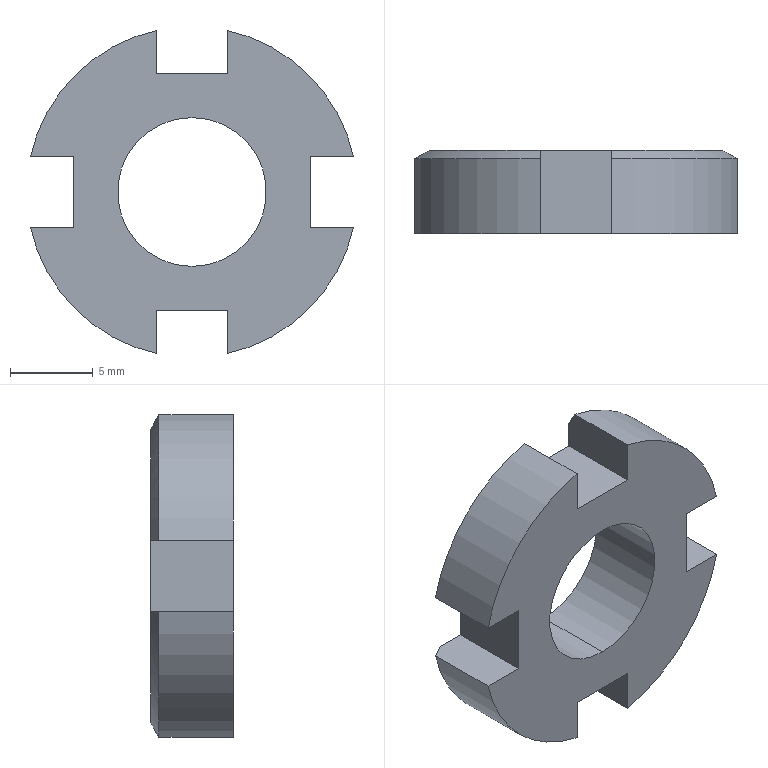Part | SolidWorks | features Chamfer 1, Extrusion 1, HoleWzd 1 | 1 solid | 24 faces | box 19.532 x 5 x 19.532 mm | volume 1006 mm3 | plane 14 | cylinder 6 | cone 4 | commonest cylinder face diameters 20 x4 9 x2
STEP:
#1=CARTESIAN_POINT('',(0.,0.,-4.5));
#2=VERTEX_POINT('',#1);
#3=CARTESIAN_POINT('',(0.,0.,4.5));
#4=VERTEX_POINT('',#3);
#5=CARTESIAN_POINT('',(0.,0.,0.));
#6=DIRECTION('',(0.,1.,0.));
#7=DIRECTION('',(0.,0.,1.));
#8=AXIS2_PLACEMENT_3D('',#5,#6,#7);
#9=CIRCLE('',#8,4.5);
#10=EDGE_CURVE('',#2,#4,#9,.T.);
#11=ORIENTED_EDGE('',*,*,#10,.F.);
#12=CARTESIAN_POINT('',(0.,5.,-4.5));
#13=VERTEX_POINT('',#12);
#14=CARTESIAN_POINT('',(0.,5.,-4.5));
#15=DIRECTION('',(0.,1.,0.));
#16=VECTOR('',#15,1000.);
#17=LINE('',#14,#16);
#18=EDGE_CURVE('',#2,#13,#17,.T.);
#19=ORIENTED_EDGE('',*,*,#18,.T.);
#20=CARTESIAN_POINT('',(0.,5.,4.5));
#21=VERTEX_POINT('',#20);
#22=CARTESIAN_POINT('',(0.,5.,0.));
#23=DIRECTION('',(0.,1.,0.));
#24=DIRECTION('',(0.,0.,1.));
#25=AXIS2_PLACEMENT_3D('',#22,#23,#24);
#26=CIRCLE('',#25,4.5);
#27=EDGE_CURVE('',#13,#21,#26,.T.);
#28=ORIENTED_EDGE('',*,*,#27,.T.);
#29=CARTESIAN_POINT('',(0.,5.,4.5));
#30=DIRECTION('',(0.,1.,0.));
#31=VECTOR('',#30,1000.);
#32=LINE('',#29,#31);
#33=EDGE_CURVE('',#4,#21,#32,.T.);
#34=ORIENTED_EDGE('',*,*,#33,.F.);
#35=EDGE_LOOP('',(#11,#19,#28,#34));
#36=FACE_OUTER_BOUND('',#35,.T.);
#37=CARTESIAN_POINT('',(0.,5.,0.));
#38=DIRECTION('',(0.,1.,0.));
#39=DIRECTION('',(0.,0.,1.));
#40=AXIS2_PLACEMENT_3D('',#37,#38,#39);
#41=CYLINDRICAL_SURFACE('',#40,4.5);
#42=ADVANCED_FACE('',(#36),#41,.F.);
#43=CARTESIAN_POINT('',(-9.766,4.5,-2.15));
#44=VERTEX_POINT('',#43);
#45=CARTESIAN_POINT('',(-9.766,0.,-2.15));
#46=VERTEX_POINT('',#45);
#47=CARTESIAN_POINT('',(-9.766,5.,-2.15));
#48=DIRECTION('',(0.,-1.,0.));
#49=VECTOR('',#48,1000.);
#50=LINE('',#47,#49);
#51=EDGE_CURVE('',#44,#46,#50,.T.);
#52=ORIENTED_EDGE('',*,*,#51,.F.);
#53=CARTESIAN_POINT('',(-2.15,4.5,-9.766));
#54=VERTEX_POINT('',#53);
#55=CARTESIAN_POINT('',(0.,4.5,0.));
#56=DIRECTION('',(0.,-1.,0.));
#57=DIRECTION('',(0.,0.,1.));
#58=AXIS2_PLACEMENT_3D('',#55,#56,#57);
#59=CIRCLE('',#58,10.);
#60=EDGE_CURVE('',#44,#54,#59,.T.);
#61=ORIENTED_EDGE('',*,*,#60,.T.);
#62=CARTESIAN_POINT('',(-2.15,0.,-9.766));
#63=VERTEX_POINT('',#62);
#64=CARTESIAN_POINT('',(-2.15,5.,-9.766));
#65=DIRECTION('',(0.,-1.,0.));
#66=VECTOR('',#65,1000.);
#67=LINE('',#64,#66);
#68=EDGE_CURVE('',#54,#63,#67,.T.);
#69=ORIENTED_EDGE('',*,*,#68,.T.);
#70=CARTESIAN_POINT('',(0.,0.,0.));
#71=DIRECTION('',(0.,1.,0.));
#72=DIRECTION('',(0.,0.,1.));
#73=AXIS2_PLACEMENT_3D('',#70,#71,#72);
#74=CIRCLE('',#73,10.);
#75=EDGE_CURVE('',#63,#46,#74,.T.);
#76=ORIENTED_EDGE('',*,*,#75,.T.);
#77=EDGE_LOOP('',(#52,#61,#69,#76));
#78=FACE_OUTER_BOUND('',#77,.T.);
#79=CARTESIAN_POINT('',(0.,5.,0.));
#80=DIRECTION('',(0.,-1.,0.));
#81=DIRECTION('',(0.,0.,-1.));
#82=AXIS2_PLACEMENT_3D('',#79,#80,#81);
#83=CYLINDRICAL_SURFACE('',#82,10.);
#84=ADVANCED_FACE('',(#78),#83,.T.);
#85=CARTESIAN_POINT('',(-8.877,5.,-2.15));
#86=VERTEX_POINT('',#85);
#87=CARTESIAN_POINT('',(-7.166,5.,-2.15));
#88=VERTEX_POINT('',#87);
#89=CARTESIAN_POINT('',(-7.166,5.,-2.15));
#90=DIRECTION('',(1.,0.,0.));
#91=VECTOR('',#90,1000.);
#92=LINE('',#89,#91);
#93=EDGE_CURVE('',#86,#88,#92,.T.);
#94=ORIENTED_EDGE('',*,*,#93,.F.);
#95=CARTESIAN_POINT('',(-8.877,5.,-2.15));
#96=CARTESIAN_POINT('',(-9.174,4.834,-2.15));
#97=CARTESIAN_POINT('',(-9.47,4.667,-2.15));
#98=CARTESIAN_POINT('',(-9.766,4.5,-2.15));
#99=B_SPLINE_CURVE_WITH_KNOTS('',3,(#95,#96,#97,#98),.UNSPECIFIED.,.F.,.F.,(4,4),(0.,0.00102),.UNSPECIFIED.);
#100=EDGE_CURVE('',#86,#44,#99,.T.);
#101=ORIENTED_EDGE('',*,*,#100,.T.);
#102=ORIENTED_EDGE('',*,*,#51,.T.);
#103=CARTESIAN_POINT('',(-7.166,0.,-2.15));
#104=VERTEX_POINT('',#103);
#105=CARTESIAN_POINT('',(-7.166,0.,-2.15));
#106=DIRECTION('',(1.,0.,0.));
#107=VECTOR('',#106,1000.);
#108=LINE('',#105,#107);
#109=EDGE_CURVE('',#46,#104,#108,.T.);
#110=ORIENTED_EDGE('',*,*,#109,.T.);
#111=CARTESIAN_POINT('',(-7.166,5.,-2.15));
#112=DIRECTION('',(0.,-1.,0.));
#113=VECTOR('',#112,1000.);
#114=LINE('',#111,#113);
#115=EDGE_CURVE('',#88,#104,#114,.T.);
#116=ORIENTED_EDGE('',*,*,#115,.F.);
#117=EDGE_LOOP('',(#94,#101,#102,#110,#116));
#118=FACE_OUTER_BOUND('',#117,.T.);
#119=CARTESIAN_POINT('',(-7.166,5.,-2.15));
#120=DIRECTION('',(0.,0.,-1.));
#121=DIRECTION('',(-1.,0.,0.));
#122=AXIS2_PLACEMENT_3D('',#119,#120,#121);
#123=PLANE('',#122);
#124=ADVANCED_FACE('',(#118),#123,.F.);
#125=CARTESIAN_POINT('',(-7.166,0.,2.15));
#126=VERTEX_POINT('',#125);
#127=CARTESIAN_POINT('',(-7.166,0.,2.15));
#128=DIRECTION('',(0.,0.,1.));
#129=VECTOR('',#128,1000.);
#130=LINE('',#127,#129);
#131=EDGE_CURVE('',#104,#126,#130,.T.);
#132=ORIENTED_EDGE('',*,*,#131,.T.);
#133=CARTESIAN_POINT('',(-7.166,5.,2.15));
#134=VERTEX_POINT('',#133);
#135=CARTESIAN_POINT('',(-7.166,5.,2.15));
#136=DIRECTION('',(0.,-1.,0.));
#137=VECTOR('',#136,1000.);
#138=LINE('',#135,#137);
#139=EDGE_CURVE('',#134,#126,#138,.T.);
#140=ORIENTED_EDGE('',*,*,#139,.F.);
#141=CARTESIAN_POINT('',(-7.166,5.,2.15));
#142=DIRECTION('',(0.,0.,1.));
#143=VECTOR('',#142,1000.);
#144=LINE('',#141,#143);
#145=EDGE_CURVE('',#88,#134,#144,.T.);
#146=ORIENTED_EDGE('',*,*,#145,.F.);
#147=ORIENTED_EDGE('',*,*,#115,.T.);
#148=EDGE_LOOP('',(#132,#140,#146,#147));
#149=FACE_OUTER_BOUND('',#148,.T.);
#150=CARTESIAN_POINT('',(-7.166,5.,2.15));
#151=DIRECTION('',(1.,0.,0.));
#152=DIRECTION('',(0.,0.,-1.));
#153=AXIS2_PLACEMENT_3D('',#150,#151,#152);
#154=PLANE('',#153);
#155=ADVANCED_FACE('',(#149),#154,.F.);
#156=CARTESIAN_POINT('',(-9.766,4.5,2.15));
#157=VERTEX_POINT('',#156);
#158=CARTESIAN_POINT('',(-9.766,0.,2.15));
#159=VERTEX_POINT('',#158);
#160=CARTESIAN_POINT('',(-9.766,5.,2.15));
#161=DIRECTION('',(0.,-1.,0.));
#162=VECTOR('',#161,1000.);
#163=LINE('',#160,#162);
#164=EDGE_CURVE('',#157,#159,#163,.T.);
#165=ORIENTED_EDGE('',*,*,#164,.F.);
#166=CARTESIAN_POINT('',(-8.877,5.,2.15));
#167=VERTEX_POINT('',#166);
#168=CARTESIAN_POINT('',(-9.766,4.5,2.15));
#169=CARTESIAN_POINT('',(-9.47,4.667,2.15));
#170=CARTESIAN_POINT('',(-9.174,4.834,2.15));
#171=CARTESIAN_POINT('',(-8.877,5.,2.15));
#172=B_SPLINE_CURVE_WITH_KNOTS('',3,(#168,#169,#170,#171),.UNSPECIFIED.,.F.,.F.,(4,4),(0.,0.00102),.UNSPECIFIED.);
#173=EDGE_CURVE('',#157,#167,#172,.T.);
#174=ORIENTED_EDGE('',*,*,#173,.T.);
#175=CARTESIAN_POINT('',(-9.766,5.,2.15));
#176=DIRECTION('',(-1.,0.,0.));
#177=VECTOR('',#176,1000.);
#178=LINE('',#175,#177);
#179=EDGE_CURVE('',#134,#167,#178,.T.);
#180=ORIENTED_EDGE('',*,*,#179,.F.);
#181=ORIENTED_EDGE('',*,*,#139,.T.);
#182=CARTESIAN_POINT('',(-9.766,0.,2.15));
#183=DIRECTION('',(-1.,0.,0.));
#184=VECTOR('',#183,1000.);
#185=LINE('',#182,#184);
#186=EDGE_CURVE('',#126,#159,#185,.T.);
#187=ORIENTED_EDGE('',*,*,#186,.T.);
#188=EDGE_LOOP('',(#165,#174,#180,#181,#187));
#189=FACE_OUTER_BOUND('',#188,.T.);
#190=CARTESIAN_POINT('',(-9.766,5.,2.15));
#191=DIRECTION('',(0.,0.,1.));
#192=DIRECTION('',(1.,0.,0.));
#193=AXIS2_PLACEMENT_3D('',#190,#191,#192);
#194=PLANE('',#193);
#195=ADVANCED_FACE('',(#189),#194,.F.);
#196=CARTESIAN_POINT('',(-2.15,4.5,9.766));
#197=VERTEX_POINT('',#196);
#198=CARTESIAN_POINT('',(-2.15,0.,9.766));
#199=VERTEX_POINT('',#198);
#200=CARTESIAN_POINT('',(-2.15,5.,9.766));
#201=DIRECTION('',(0.,-1.,0.));
#202=VECTOR('',#201,1000.);
#203=LINE('',#200,#202);
#204=EDGE_CURVE('',#197,#199,#203,.T.);
#205=ORIENTED_EDGE('',*,*,#204,.F.);
#206=CARTESIAN_POINT('',(0.,4.5,0.));
#207=DIRECTION('',(0.,-1.,0.));
#208=DIRECTION('',(0.,0.,1.));
#209=AXIS2_PLACEMENT_3D('',#206,#207,#208);
#210=CIRCLE('',#209,10.);
#211=EDGE_CURVE('',#197,#157,#210,.T.);
#212=ORIENTED_EDGE('',*,*,#211,.T.);
#213=ORIENTED_EDGE('',*,*,#164,.T.);
#214=CARTESIAN_POINT('',(0.,0.,0.));
#215=DIRECTION('',(0.,1.,0.));
#216=DIRECTION('',(0.,0.,1.));
#217=AXIS2_PLACEMENT_3D('',#214,#215,#216);
#218=CIRCLE('',#217,10.);
#219=EDGE_CURVE('',#159,#199,#218,.T.);
#220=ORIENTED_EDGE('',*,*,#219,.T.);
#221=EDGE_LOOP('',(#205,#212,#213,#220));
#222=FACE_OUTER_BOUND('',#221,.T.);
#223=CARTESIAN_POINT('',(0.,5.,0.));
#224=DIRECTION('',(0.,-1.,0.));
#225=DIRECTION('',(0.,0.,-1.));
#226=AXIS2_PLACEMENT_3D('',#223,#224,#225);
#227=CYLINDRICAL_SURFACE('',#226,10.);
#228=ADVANCED_FACE('',(#222),#227,.T.);
#229=CARTESIAN_POINT('',(-2.15,5.,8.877));
#230=VERTEX_POINT('',#229);
#231=CARTESIAN_POINT('',(-2.15,5.,7.166));
#232=VERTEX_POINT('',#231);
#233=CARTESIAN_POINT('',(-2.15,5.,7.166));
#234=DIRECTION('',(0.,0.,-1.));
#235=VECTOR('',#234,1000.);
#236=LINE('',#233,#235);
#237=EDGE_CURVE('',#230,#232,#236,.T.);
#238=ORIENTED_EDGE('',*,*,#237,.F.);
#239=CARTESIAN_POINT('',(-2.15,5.,8.877));
#240=CARTESIAN_POINT('',(-2.15,4.834,9.174));
#241=CARTESIAN_POINT('',(-2.15,4.667,9.47));
#242=CARTESIAN_POINT('',(-2.15,4.5,9.766));
#243=B_SPLINE_CURVE_WITH_KNOTS('',3,(#239,#240,#241,#242),.UNSPECIFIED.,.F.,.F.,(4,4),(0.,0.00102),.UNSPECIFIED.);
#244=EDGE_CURVE('',#230,#197,#243,.T.);
#245=ORIENTED_EDGE('',*,*,#244,.T.);
#246=ORIENTED_EDGE('',*,*,#204,.T.);
#247=CARTESIAN_POINT('',(-2.15,0.,7.166));
#248=VERTEX_POINT('',#247);
#249=CARTESIAN_POINT('',(-2.15,0.,7.166));
#250=DIRECTION('',(0.,0.,-1.));
#251=VECTOR('',#250,1000.);
#252=LINE('',#249,#251);
#253=EDGE_CURVE('',#199,#248,#252,.T.);
#254=ORIENTED_EDGE('',*,*,#253,.T.);
#255=CARTESIAN_POINT('',(-2.15,5.,7.166));
#256=DIRECTION('',(0.,-1.,0.));
#257=VECTOR('',#256,1000.);
#258=LINE('',#255,#257);
#259=EDGE_CURVE('',#232,#248,#258,.T.);
#260=ORIENTED_EDGE('',*,*,#259,.F.);
#261=EDGE_LOOP('',(#238,#245,#246,#254,#260));
#262=FACE_OUTER_BOUND('',#261,.T.);
#263=CARTESIAN_POINT('',(-2.15,5.,7.166));
#264=DIRECTION('',(-1.,0.,0.));
#265=DIRECTION('',(0.,0.,1.));
#266=AXIS2_PLACEMENT_3D('',#263,#264,#265);
#267=PLANE('',#266);
#268=ADVANCED_FACE('',(#262),#267,.F.);
#269=CARTESIAN_POINT('',(2.15,0.,7.166));
#270=VERTEX_POINT('',#269);
#271=CARTESIAN_POINT('',(2.15,0.,7.166));
#272=DIRECTION('',(1.,0.,0.));
#273=VECTOR('',#272,1000.);
#274=LINE('',#271,#273);
#275=EDGE_CURVE('',#248,#270,#274,.T.);
#276=ORIENTED_EDGE('',*,*,#275,.T.);
#277=CARTESIAN_POINT('',(2.15,5.,7.166));
#278=VERTEX_POINT('',#277);
#279=CARTESIAN_POINT('',(2.15,5.,7.166));
#280=DIRECTION('',(0.,-1.,0.));
#281=VECTOR('',#280,1000.);
#282=LINE('',#279,#281);
#283=EDGE_CURVE('',#278,#270,#282,.T.);
#284=ORIENTED_EDGE('',*,*,#283,.F.);
#285=CARTESIAN_POINT('',(2.15,5.,7.166));
#286=DIRECTION('',(1.,0.,0.));
#287=VECTOR('',#286,1000.);
#288=LINE('',#285,#287);
#289=EDGE_CURVE('',#232,#278,#288,.T.);
#290=ORIENTED_EDGE('',*,*,#289,.F.);
#291=ORIENTED_EDGE('',*,*,#259,.T.);
#292=EDGE_LOOP('',(#276,#284,#290,#291));
#293=FACE_OUTER_BOUND('',#292,.T.);
#294=CARTESIAN_POINT('',(2.15,5.,7.166));
#295=DIRECTION('',(0.,0.,-1.));
#296=DIRECTION('',(-1.,0.,0.));
#297=AXIS2_PLACEMENT_3D('',#294,#295,#296);
#298=PLANE('',#297);
#299=ADVANCED_FACE('',(#293),#298,.F.);
#300=CARTESIAN_POINT('',(2.15,4.5,9.766));
#301=VERTEX_POINT('',#300);
#302=CARTESIAN_POINT('',(2.15,0.,9.766));
#303=VERTEX_POINT('',#302);
#304=CARTESIAN_POINT('',(2.15,5.,9.766));
#305=DIRECTION('',(0.,-1.,0.));
#306=VECTOR('',#305,1000.);
#307=LINE('',#304,#306);
#308=EDGE_CURVE('',#301,#303,#307,.T.);
#309=ORIENTED_EDGE('',*,*,#308,.F.);
#310=CARTESIAN_POINT('',(2.15,5.,8.877));
#311=VERTEX_POINT('',#310);
#312=CARTESIAN_POINT('',(2.15,4.5,9.766));
#313=CARTESIAN_POINT('',(2.15,4.667,9.47));
#314=CARTESIAN_POINT('',(2.15,4.834,9.174));
#315=CARTESIAN_POINT('',(2.15,5.,8.877));
#316=B_SPLINE_CURVE_WITH_KNOTS('',3,(#312,#313,#314,#315),.UNSPECIFIED.,.F.,.F.,(4,4),(0.,0.00102),.UNSPECIFIED.);
#317=EDGE_CURVE('',#301,#311,#316,.T.);
#318=ORIENTED_EDGE('',*,*,#317,.T.);
#319=CARTESIAN_POINT('',(2.15,5.,9.766));
#320=DIRECTION('',(0.,0.,1.));
#321=VECTOR('',#320,1000.);
#322=LINE('',#319,#321);
#323=EDGE_CURVE('',#278,#311,#322,.T.);
#324=ORIENTED_EDGE('',*,*,#323,.F.);
#325=ORIENTED_EDGE('',*,*,#283,.T.);
#326=CARTESIAN_POINT('',(2.15,0.,9.766));
#327=DIRECTION('',(0.,0.,1.));
#328=VECTOR('',#327,1000.);
#329=LINE('',#326,#328);
#330=EDGE_CURVE('',#270,#303,#329,.T.);
#331=ORIENTED_EDGE('',*,*,#330,.T.);
#332=EDGE_LOOP('',(#309,#318,#324,#325,#331));
#333=FACE_OUTER_BOUND('',#332,.T.);
#334=CARTESIAN_POINT('',(2.15,5.,9.766));
#335=DIRECTION('',(1.,0.,0.));
#336=DIRECTION('',(0.,0.,-1.));
#337=AXIS2_PLACEMENT_3D('',#334,#335,#336);
#338=PLANE('',#337);
#339=ADVANCED_FACE('',(#333),#338,.F.);
#340=CARTESIAN_POINT('',(9.766,4.5,2.15));
#341=VERTEX_POINT('',#340);
#342=CARTESIAN_POINT('',(9.766,0.,2.15));
#343=VERTEX_POINT('',#342);
#344=CARTESIAN_POINT('',(9.766,5.,2.15));
#345=DIRECTION('',(0.,-1.,0.));
#346=VECTOR('',#345,1000.);
#347=LINE('',#344,#346);
#348=EDGE_CURVE('',#341,#343,#347,.T.);
#349=ORIENTED_EDGE('',*,*,#348,.F.);
#350=CARTESIAN_POINT('',(0.,4.5,0.));
#351=DIRECTION('',(0.,-1.,0.));
#352=DIRECTION('',(0.,0.,1.));
#353=AXIS2_PLACEMENT_3D('',#350,#351,#352);
#354=CIRCLE('',#353,10.);
#355=EDGE_CURVE('',#341,#301,#354,.T.);
#356=ORIENTED_EDGE('',*,*,#355,.T.);
#357=ORIENTED_EDGE('',*,*,#308,.T.);
#358=CARTESIAN_POINT('',(0.,0.,0.));
#359=DIRECTION('',(0.,1.,0.));
#360=DIRECTION('',(0.,0.,1.));
#361=AXIS2_PLACEMENT_3D('',#358,#359,#360);
#362=CIRCLE('',#361,10.);
#363=EDGE_CURVE('',#303,#343,#362,.T.);
#364=ORIENTED_EDGE('',*,*,#363,.T.);
#365=EDGE_LOOP('',(#349,#356,#357,#364));
#366=FACE_OUTER_BOUND('',#365,.T.);
#367=CARTESIAN_POINT('',(0.,5.,0.));
#368=DIRECTION('',(0.,-1.,0.));
#369=DIRECTION('',(0.,0.,-1.));
#370=AXIS2_PLACEMENT_3D('',#367,#368,#369);
#371=CYLINDRICAL_SURFACE('',#370,10.);
#372=ADVANCED_FACE('',(#366),#371,.T.);
#373=CARTESIAN_POINT('',(8.877,5.,2.15));
#374=VERTEX_POINT('',#373);
#375=CARTESIAN_POINT('',(7.166,5.,2.15));
#376=VERTEX_POINT('',#375);
#377=CARTESIAN_POINT('',(7.166,5.,2.15));
#378=DIRECTION('',(-1.,0.,0.));
#379=VECTOR('',#378,1000.);
#380=LINE('',#377,#379);
#381=EDGE_CURVE('',#374,#376,#380,.T.);
#382=ORIENTED_EDGE('',*,*,#381,.F.);
#383=CARTESIAN_POINT('',(8.877,5.,2.15));
#384=CARTESIAN_POINT('',(9.174,4.834,2.15));
#385=CARTESIAN_POINT('',(9.47,4.667,2.15));
#386=CARTESIAN_POINT('',(9.766,4.5,2.15));
#387=B_SPLINE_CURVE_WITH_KNOTS('',3,(#383,#384,#385,#386),.UNSPECIFIED.,.F.,.F.,(4,4),(0.,0.00102),.UNSPECIFIED.);
#388=EDGE_CURVE('',#374,#341,#387,.T.);
#389=ORIENTED_EDGE('',*,*,#388,.T.);
#390=ORIENTED_EDGE('',*,*,#348,.T.);
#391=CARTESIAN_POINT('',(7.166,0.,2.15));
#392=VERTEX_POINT('',#391);
#393=CARTESIAN_POINT('',(7.166,0.,2.15));
#394=DIRECTION('',(-1.,0.,0.));
#395=VECTOR('',#394,1000.);
#396=LINE('',#393,#395);
#397=EDGE_CURVE('',#343,#392,#396,.T.);
#398=ORIENTED_EDGE('',*,*,#397,.T.);
#399=CARTESIAN_POINT('',(7.166,5.,2.15));
#400=DIRECTION('',(0.,-1.,0.));
#401=VECTOR('',#400,1000.);
#402=LINE('',#399,#401);
#403=EDGE_CURVE('',#376,#392,#402,.T.);
#404=ORIENTED_EDGE('',*,*,#403,.F.);
#405=EDGE_LOOP('',(#382,#389,#390,#398,#404));
#406=FACE_OUTER_BOUND('',#405,.T.);
#407=CARTESIAN_POINT('',(7.166,5.,2.15));
#408=DIRECTION('',(0.,0.,1.));
#409=DIRECTION('',(1.,0.,0.));
#410=AXIS2_PLACEMENT_3D('',#407,#408,#409);
#411=PLANE('',#410);
#412=ADVANCED_FACE('',(#406),#411,.F.);
#413=CARTESIAN_POINT('',(7.166,0.,-2.15));
#414=VERTEX_POINT('',#413);
#415=CARTESIAN_POINT('',(7.166,0.,-2.15));
#416=DIRECTION('',(0.,0.,-1.));
#417=VECTOR('',#416,1000.);
#418=LINE('',#415,#417);
#419=EDGE_CURVE('',#392,#414,#418,.T.);
#420=ORIENTED_EDGE('',*,*,#419,.T.);
#421=CARTESIAN_POINT('',(7.166,5.,-2.15));
#422=VERTEX_POINT('',#421);
#423=CARTESIAN_POINT('',(7.166,5.,-2.15));
#424=DIRECTION('',(0.,-1.,0.));
#425=VECTOR('',#424,1000.);
#426=LINE('',#423,#425);
#427=EDGE_CURVE('',#422,#414,#426,.T.);
#428=ORIENTED_EDGE('',*,*,#427,.F.);
#429=CARTESIAN_POINT('',(7.166,5.,-2.15));
#430=DIRECTION('',(0.,0.,-1.));
#431=VECTOR('',#430,1000.);
#432=LINE('',#429,#431);
#433=EDGE_CURVE('',#376,#422,#432,.T.);
#434=ORIENTED_EDGE('',*,*,#433,.F.);
#435=ORIENTED_EDGE('',*,*,#403,.T.);
#436=EDGE_LOOP('',(#420,#428,#434,#435));
#437=FACE_OUTER_BOUND('',#436,.T.);
#438=CARTESIAN_POINT('',(7.166,5.,-2.15));
#439=DIRECTION('',(-1.,0.,0.));
#440=DIRECTION('',(0.,0.,1.));
#441=AXIS2_PLACEMENT_3D('',#438,#439,#440);
#442=PLANE('',#441);
#443=ADVANCED_FACE('',(#437),#442,.F.);
#444=CARTESIAN_POINT('',(9.766,4.5,-2.15));
#445=VERTEX_POINT('',#444);
#446=CARTESIAN_POINT('',(9.766,0.,-2.15));
#447=VERTEX_POINT('',#446);
#448=CARTESIAN_POINT('',(9.766,5.,-2.15));
#449=DIRECTION('',(0.,-1.,0.));
#450=VECTOR('',#449,1000.);
#451=LINE('',#448,#450);
#452=EDGE_CURVE('',#445,#447,#451,.T.);
#453=ORIENTED_EDGE('',*,*,#452,.F.);
#454=CARTESIAN_POINT('',(8.877,5.,-2.15));
#455=VERTEX_POINT('',#454);
#456=CARTESIAN_POINT('',(9.766,4.5,-2.15));
#457=CARTESIAN_POINT('',(9.47,4.667,-2.15));
#458=CARTESIAN_POINT('',(9.174,4.834,-2.15));
#459=CARTESIAN_POINT('',(8.877,5.,-2.15));
#460=B_SPLINE_CURVE_WITH_KNOTS('',3,(#456,#457,#458,#459),.UNSPECIFIED.,.F.,.F.,(4,4),(0.,0.00102),.UNSPECIFIED.);
#461=EDGE_CURVE('',#445,#455,#460,.T.);
#462=ORIENTED_EDGE('',*,*,#461,.T.);
#463=CARTESIAN_POINT('',(9.766,5.,-2.15));
#464=DIRECTION('',(1.,0.,0.));
#465=VECTOR('',#464,1000.);
#466=LINE('',#463,#465);
#467=EDGE_CURVE('',#422,#455,#466,.T.);
#468=ORIENTED_EDGE('',*,*,#467,.F.);
#469=ORIENTED_EDGE('',*,*,#427,.T.);
#470=CARTESIAN_POINT('',(9.766,0.,-2.15));
#471=DIRECTION('',(1.,0.,0.));
#472=VECTOR('',#471,1000.);
#473=LINE('',#470,#472);
#474=EDGE_CURVE('',#414,#447,#473,.T.);
#475=ORIENTED_EDGE('',*,*,#474,.T.);
#476=EDGE_LOOP('',(#453,#462,#468,#469,#475));
#477=FACE_OUTER_BOUND('',#476,.T.);
#478=CARTESIAN_POINT('',(9.766,5.,-2.15));
#479=DIRECTION('',(0.,0.,-1.));
#480=DIRECTION('',(-1.,0.,0.));
#481=AXIS2_PLACEMENT_3D('',#478,#479,#480);
#482=PLANE('',#481);
#483=ADVANCED_FACE('',(#477),#482,.F.);
#484=CARTESIAN_POINT('',(2.15,4.5,-9.766));
#485=VERTEX_POINT('',#484);
#486=CARTESIAN_POINT('',(2.15,0.,-9.766));
#487=VERTEX_POINT('',#486);
#488=CARTESIAN_POINT('',(2.15,5.,-9.766));
#489=DIRECTION('',(0.,-1.,0.));
#490=VECTOR('',#489,1000.);
#491=LINE('',#488,#490);
#492=EDGE_CURVE('',#485,#487,#491,.T.);
#493=ORIENTED_EDGE('',*,*,#492,.F.);
#494=CARTESIAN_POINT('',(0.,4.5,0.));
#495=DIRECTION('',(0.,-1.,0.));
#496=DIRECTION('',(0.,0.,1.));
#497=AXIS2_PLACEMENT_3D('',#494,#495,#496);
#498=CIRCLE('',#497,10.);
#499=EDGE_CURVE('',#485,#445,#498,.T.);
#500=ORIENTED_EDGE('',*,*,#499,.T.);
#501=ORIENTED_EDGE('',*,*,#452,.T.);
#502=CARTESIAN_POINT('',(0.,0.,0.));
#503=DIRECTION('',(0.,1.,0.));
#504=DIRECTION('',(0.,0.,1.));
#505=AXIS2_PLACEMENT_3D('',#502,#503,#504);
#506=CIRCLE('',#505,10.);
#507=EDGE_CURVE('',#447,#487,#506,.T.);
#508=ORIENTED_EDGE('',*,*,#507,.T.);
#509=EDGE_LOOP('',(#493,#500,#501,#508));
#510=FACE_OUTER_BOUND('',#509,.T.);
#511=CARTESIAN_POINT('',(0.,5.,0.));
#512=DIRECTION('',(0.,-1.,0.));
#513=DIRECTION('',(0.,0.,-1.));
#514=AXIS2_PLACEMENT_3D('',#511,#512,#513);
#515=CYLINDRICAL_SURFACE('',#514,10.);
#516=ADVANCED_FACE('',(#510),#515,.T.);
#517=CARTESIAN_POINT('',(2.15,5.,-8.877));
#518=VERTEX_POINT('',#517);
#519=CARTESIAN_POINT('',(2.15,5.,-7.166));
#520=VERTEX_POINT('',#519);
#521=CARTESIAN_POINT('',(2.15,5.,-7.166));
#522=DIRECTION('',(0.,0.,1.));
#523=VECTOR('',#522,1000.);
#524=LINE('',#521,#523);
#525=EDGE_CURVE('',#518,#520,#524,.T.);
#526=ORIENTED_EDGE('',*,*,#525,.F.);
#527=CARTESIAN_POINT('',(2.15,5.,-8.877));
#528=CARTESIAN_POINT('',(2.15,4.834,-9.174));
#529=CARTESIAN_POINT('',(2.15,4.667,-9.47));
#530=CARTESIAN_POINT('',(2.15,4.5,-9.766));
#531=B_SPLINE_CURVE_WITH_KNOTS('',3,(#527,#528,#529,#530),.UNSPECIFIED.,.F.,.F.,(4,4),(0.,0.00102),.UNSPECIFIED.);
#532=EDGE_CURVE('',#518,#485,#531,.T.);
#533=ORIENTED_EDGE('',*,*,#532,.T.);
#534=ORIENTED_EDGE('',*,*,#492,.T.);
#535=CARTESIAN_POINT('',(2.15,0.,-7.166));
#536=VERTEX_POINT('',#535);
#537=CARTESIAN_POINT('',(2.15,0.,-7.166));
#538=DIRECTION('',(0.,0.,1.));
#539=VECTOR('',#538,1000.);
#540=LINE('',#537,#539);
#541=EDGE_CURVE('',#487,#536,#540,.T.);
#542=ORIENTED_EDGE('',*,*,#541,.T.);
#543=CARTESIAN_POINT('',(2.15,5.,-7.166));
#544=DIRECTION('',(0.,-1.,0.));
#545=VECTOR('',#544,1000.);
#546=LINE('',#543,#545);
#547=EDGE_CURVE('',#520,#536,#546,.T.);
#548=ORIENTED_EDGE('',*,*,#547,.F.);
#549=EDGE_LOOP('',(#526,#533,#534,#542,#548));
#550=FACE_OUTER_BOUND('',#549,.T.);
#551=CARTESIAN_POINT('',(2.15,5.,-7.166));
#552=DIRECTION('',(1.,0.,0.));
#553=DIRECTION('',(0.,0.,-1.));
#554=AXIS2_PLACEMENT_3D('',#551,#552,#553);
#555=PLANE('',#554);
#556=ADVANCED_FACE('',(#550),#555,.F.);
#557=CARTESIAN_POINT('',(-2.15,0.,-7.166));
#558=VERTEX_POINT('',#557);
#559=CARTESIAN_POINT('',(-2.15,0.,-7.166));
#560=DIRECTION('',(-1.,0.,0.));
#561=VECTOR('',#560,1000.);
#562=LINE('',#559,#561);
#563=EDGE_CURVE('',#536,#558,#562,.T.);
#564=ORIENTED_EDGE('',*,*,#563,.T.);
#565=CARTESIAN_POINT('',(-2.15,5.,-7.166));
#566=VERTEX_POINT('',#565);
#567=CARTESIAN_POINT('',(-2.15,5.,-7.166));
#568=DIRECTION('',(0.,-1.,0.));
#569=VECTOR('',#568,1000.);
#570=LINE('',#567,#569);
#571=EDGE_CURVE('',#566,#558,#570,.T.);
#572=ORIENTED_EDGE('',*,*,#571,.F.);
#573=CARTESIAN_POINT('',(-2.15,5.,-7.166));
#574=DIRECTION('',(-1.,0.,0.));
#575=VECTOR('',#574,1000.);
#576=LINE('',#573,#575);
#577=EDGE_CURVE('',#520,#566,#576,.T.);
#578=ORIENTED_EDGE('',*,*,#577,.F.);
#579=ORIENTED_EDGE('',*,*,#547,.T.);
#580=EDGE_LOOP('',(#564,#572,#578,#579));
#581=FACE_OUTER_BOUND('',#580,.T.);
#582=CARTESIAN_POINT('',(-2.15,5.,-7.166));
#583=DIRECTION('',(0.,0.,1.));
#584=DIRECTION('',(1.,0.,0.));
#585=AXIS2_PLACEMENT_3D('',#582,#583,#584);
#586=PLANE('',#585);
#587=ADVANCED_FACE('',(#581),#586,.F.);
#588=ORIENTED_EDGE('',*,*,#68,.F.);
#589=CARTESIAN_POINT('',(-2.15,5.,-8.877));
#590=VERTEX_POINT('',#589);
#591=CARTESIAN_POINT('',(-2.15,4.5,-9.766));
#592=CARTESIAN_POINT('',(-2.15,4.667,-9.47));
#593=CARTESIAN_POINT('',(-2.15,4.834,-9.174));
#594=CARTESIAN_POINT('',(-2.15,5.,-8.877));
#595=B_SPLINE_CURVE_WITH_KNOTS('',3,(#591,#592,#593,#594),.UNSPECIFIED.,.F.,.F.,(4,4),(0.,0.00102),.UNSPECIFIED.);
#596=EDGE_CURVE('',#54,#590,#595,.T.);
#597=ORIENTED_EDGE('',*,*,#596,.T.);
#598=CARTESIAN_POINT('',(-2.15,5.,-9.766));
#599=DIRECTION('',(0.,0.,-1.));
#600=VECTOR('',#599,1000.);
#601=LINE('',#598,#600);
#602=EDGE_CURVE('',#566,#590,#601,.T.);
#603=ORIENTED_EDGE('',*,*,#602,.F.);
#604=ORIENTED_EDGE('',*,*,#571,.T.);
#605=CARTESIAN_POINT('',(-2.15,0.,-9.766));
#606=DIRECTION('',(0.,0.,-1.));
#607=VECTOR('',#606,1000.);
#608=LINE('',#605,#607);
#609=EDGE_CURVE('',#558,#63,#608,.T.);
#610=ORIENTED_EDGE('',*,*,#609,.T.);
#611=EDGE_LOOP('',(#588,#597,#603,#604,#610));
#612=FACE_OUTER_BOUND('',#611,.T.);
#613=CARTESIAN_POINT('',(-2.15,5.,-9.766));
#614=DIRECTION('',(-1.,0.,0.));
#615=DIRECTION('',(0.,0.,1.));
#616=AXIS2_PLACEMENT_3D('',#613,#614,#615);
#617=PLANE('',#616);
#618=ADVANCED_FACE('',(#612),#617,.F.);
#619=CARTESIAN_POINT('',(0.,5.,0.));
#620=DIRECTION('',(0.,1.,0.));
#621=DIRECTION('',(0.,0.,1.));
#622=AXIS2_PLACEMENT_3D('',#619,#620,#621);
#623=CIRCLE('',#622,4.5);
#624=EDGE_CURVE('',#21,#13,#623,.T.);
#625=ORIENTED_EDGE('',*,*,#624,.F.);
#626=ORIENTED_EDGE('',*,*,#27,.F.);
#627=EDGE_LOOP('',(#625,#626));
#628=FACE_BOUND('',#627,.T.);
#629=ORIENTED_EDGE('',*,*,#602,.T.);
#630=CARTESIAN_POINT('',(0.,5.,0.));
#631=DIRECTION('',(0.,1.,0.));
#632=DIRECTION('',(0.,0.,1.));
#633=AXIS2_PLACEMENT_3D('',#630,#631,#632);
#634=CIRCLE('',#633,9.134);
#635=EDGE_CURVE('',#590,#86,#634,.T.);
#636=ORIENTED_EDGE('',*,*,#635,.T.);
#637=ORIENTED_EDGE('',*,*,#93,.T.);
#638=ORIENTED_EDGE('',*,*,#145,.T.);
#639=ORIENTED_EDGE('',*,*,#179,.T.);
#640=CARTESIAN_POINT('',(0.,5.,0.));
#641=DIRECTION('',(0.,1.,0.));
#642=DIRECTION('',(0.,0.,1.));
#643=AXIS2_PLACEMENT_3D('',#640,#641,#642);
#644=CIRCLE('',#643,9.134);
#645=EDGE_CURVE('',#167,#230,#644,.T.);
#646=ORIENTED_EDGE('',*,*,#645,.T.);
#647=ORIENTED_EDGE('',*,*,#237,.T.);
#648=ORIENTED_EDGE('',*,*,#289,.T.);
#649=ORIENTED_EDGE('',*,*,#323,.T.);
#650=CARTESIAN_POINT('',(0.,5.,0.));
#651=DIRECTION('',(0.,1.,0.));
#652=DIRECTION('',(0.,0.,1.));
#653=AXIS2_PLACEMENT_3D('',#650,#651,#652);
#654=CIRCLE('',#653,9.134);
#655=EDGE_CURVE('',#311,#374,#654,.T.);
#656=ORIENTED_EDGE('',*,*,#655,.T.);
#657=ORIENTED_EDGE('',*,*,#381,.T.);
#658=ORIENTED_EDGE('',*,*,#433,.T.);
#659=ORIENTED_EDGE('',*,*,#467,.T.);
#660=CARTESIAN_POINT('',(0.,5.,0.));
#661=DIRECTION('',(0.,1.,0.));
#662=DIRECTION('',(0.,0.,1.));
#663=AXIS2_PLACEMENT_3D('',#660,#661,#662);
#664=CIRCLE('',#663,9.134);
#665=EDGE_CURVE('',#455,#518,#664,.T.);
#666=ORIENTED_EDGE('',*,*,#665,.T.);
#667=ORIENTED_EDGE('',*,*,#525,.T.);
#668=ORIENTED_EDGE('',*,*,#577,.T.);
#669=EDGE_LOOP('',(#629,#636,#637,#638,#639,#646,#647,#648,#649,#656,#657,#658,#659,#666,#667,#668));
#670=FACE_OUTER_BOUND('',#669,.T.);
#671=CARTESIAN_POINT('',(0.,5.,0.));
#672=DIRECTION('',(0.,1.,0.));
#673=DIRECTION('',(0.,0.,1.));
#674=AXIS2_PLACEMENT_3D('',#671,#672,#673);
#675=PLANE('',#674);
#676=ADVANCED_FACE('',(#628,#670),#675,.T.);
#677=CARTESIAN_POINT('',(0.,0.,0.));
#678=DIRECTION('',(0.,1.,0.));
#679=DIRECTION('',(0.,0.,1.));
#680=AXIS2_PLACEMENT_3D('',#677,#678,#679);
#681=CIRCLE('',#680,4.5);
#682=EDGE_CURVE('',#4,#2,#681,.T.);
#683=ORIENTED_EDGE('',*,*,#682,.T.);
#684=ORIENTED_EDGE('',*,*,#10,.T.);
#685=EDGE_LOOP('',(#683,#684));
#686=FACE_BOUND('',#685,.T.);
#687=ORIENTED_EDGE('',*,*,#75,.F.);
#688=ORIENTED_EDGE('',*,*,#609,.F.);
#689=ORIENTED_EDGE('',*,*,#563,.F.);
#690=ORIENTED_EDGE('',*,*,#541,.F.);
#691=ORIENTED_EDGE('',*,*,#507,.F.);
#692=ORIENTED_EDGE('',*,*,#474,.F.);
#693=ORIENTED_EDGE('',*,*,#419,.F.);
#694=ORIENTED_EDGE('',*,*,#397,.F.);
#695=ORIENTED_EDGE('',*,*,#363,.F.);
#696=ORIENTED_EDGE('',*,*,#330,.F.);
#697=ORIENTED_EDGE('',*,*,#275,.F.);
#698=ORIENTED_EDGE('',*,*,#253,.F.);
#699=ORIENTED_EDGE('',*,*,#219,.F.);
#700=ORIENTED_EDGE('',*,*,#186,.F.);
#701=ORIENTED_EDGE('',*,*,#131,.F.);
#702=ORIENTED_EDGE('',*,*,#109,.F.);
#703=EDGE_LOOP('',(#687,#688,#689,#690,#691,#692,#693,#694,#695,#696,#697,#698,#699,#700,#701,#702));
#704=FACE_OUTER_BOUND('',#703,.T.);
#705=CARTESIAN_POINT('',(0.,0.,0.));
#706=DIRECTION('',(0.,1.,0.));
#707=DIRECTION('',(0.,0.,1.));
#708=AXIS2_PLACEMENT_3D('',#705,#706,#707);
#709=PLANE('',#708);
#710=ADVANCED_FACE('',(#686,#704),#709,.F.);
#711=ORIENTED_EDGE('',*,*,#18,.F.);
#712=ORIENTED_EDGE('',*,*,#682,.F.);
#713=ORIENTED_EDGE('',*,*,#33,.T.);
#714=ORIENTED_EDGE('',*,*,#624,.T.);
#715=EDGE_LOOP('',(#711,#712,#713,#714));
#716=FACE_OUTER_BOUND('',#715,.T.);
#717=CARTESIAN_POINT('',(0.,5.,0.));
#718=DIRECTION('',(0.,1.,0.));
#719=DIRECTION('',(0.,0.,1.));
#720=AXIS2_PLACEMENT_3D('',#717,#718,#719);
#721=CYLINDRICAL_SURFACE('',#720,4.5);
#722=ADVANCED_FACE('',(#716),#721,.F.);
#723=ORIENTED_EDGE('',*,*,#596,.F.);
#724=ORIENTED_EDGE('',*,*,#60,.F.);
#725=ORIENTED_EDGE('',*,*,#100,.F.);
#726=ORIENTED_EDGE('',*,*,#635,.F.);
#727=EDGE_LOOP('',(#723,#724,#725,#726));
#728=FACE_OUTER_BOUND('',#727,.T.);
#729=CARTESIAN_POINT('',(0.,5.,0.));
#730=DIRECTION('',(0.,-1.,0.));
#731=DIRECTION('',(0.,0.,-1.));
#732=AXIS2_PLACEMENT_3D('',#729,#730,#731);
#733=CONICAL_SURFACE('',#732,9.134,1.047);
#734=ADVANCED_FACE('',(#728),#733,.T.);
#735=ORIENTED_EDGE('',*,*,#461,.F.);
#736=ORIENTED_EDGE('',*,*,#499,.F.);
#737=ORIENTED_EDGE('',*,*,#532,.F.);
#738=ORIENTED_EDGE('',*,*,#665,.F.);
#739=EDGE_LOOP('',(#735,#736,#737,#738));
#740=FACE_OUTER_BOUND('',#739,.T.);
#741=CARTESIAN_POINT('',(0.,5.,0.));
#742=DIRECTION('',(0.,-1.,0.));
#743=DIRECTION('',(0.,0.,-1.));
#744=AXIS2_PLACEMENT_3D('',#741,#742,#743);
#745=CONICAL_SURFACE('',#744,9.134,1.047);
#746=ADVANCED_FACE('',(#740),#745,.T.);
#747=ORIENTED_EDGE('',*,*,#317,.F.);
#748=ORIENTED_EDGE('',*,*,#355,.F.);
#749=ORIENTED_EDGE('',*,*,#388,.F.);
#750=ORIENTED_EDGE('',*,*,#655,.F.);
#751=EDGE_LOOP('',(#747,#748,#749,#750));
#752=FACE_OUTER_BOUND('',#751,.T.);
#753=CARTESIAN_POINT('',(0.,5.,0.));
#754=DIRECTION('',(0.,-1.,0.));
#755=DIRECTION('',(0.,0.,-1.));
#756=AXIS2_PLACEMENT_3D('',#753,#754,#755);
#757=CONICAL_SURFACE('',#756,9.134,1.047);
#758=ADVANCED_FACE('',(#752),#757,.T.);
#759=ORIENTED_EDGE('',*,*,#173,.F.);
#760=ORIENTED_EDGE('',*,*,#211,.F.);
#761=ORIENTED_EDGE('',*,*,#244,.F.);
#762=ORIENTED_EDGE('',*,*,#645,.F.);
#763=EDGE_LOOP('',(#759,#760,#761,#762));
#764=FACE_OUTER_BOUND('',#763,.T.);
#765=CARTESIAN_POINT('',(0.,5.,0.));
#766=DIRECTION('',(0.,-1.,0.));
#767=DIRECTION('',(0.,0.,-1.));
#768=AXIS2_PLACEMENT_3D('',#765,#766,#767);
#769=CONICAL_SURFACE('',#768,9.134,1.047);
#770=ADVANCED_FACE('',(#764),#769,.T.);
#771=CLOSED_SHELL('',(#42,#84,#124,#155,#195,#228,#268,#299,#339,#372,#412,#443,#483,#516,#556,#587,#618,#676,#710,#722,#734,#746,#758,#770));
#772=MANIFOLD_SOLID_BREP('',#771);
#773=CARTESIAN_POINT('',(0.,0.,0.));
#774=DIRECTION('',(0.,0.,1.));
#775=DIRECTION('',(1.,0.,0.));
#776=AXIS2_PLACEMENT_3D('',#773,#774,#775);
#777=(LENGTH_UNIT()NAMED_UNIT(*)SI_UNIT(.MILLI.,.METRE.));
#778=UNCERTAINTY_MEASURE_WITH_UNIT(LENGTH_MEASURE(0.00001),#777,'','');
#779=(NAMED_UNIT(*)PLANE_ANGLE_UNIT()SI_UNIT($,.RADIAN.));
#780=(NAMED_UNIT(*)SI_UNIT($,.STERADIAN.)SOLID_ANGLE_UNIT());
#781=(GEOMETRIC_REPRESENTATION_CONTEXT(3)GLOBAL_UNCERTAINTY_ASSIGNED_CONTEXT((#778))GLOBAL_UNIT_ASSIGNED_CONTEXT((#777,#779,#780))REPRESENTATION_CONTEXT('',''));
#782=ADVANCED_BREP_SHAPE_REPRESENTATION('',(#772,#776),#781);